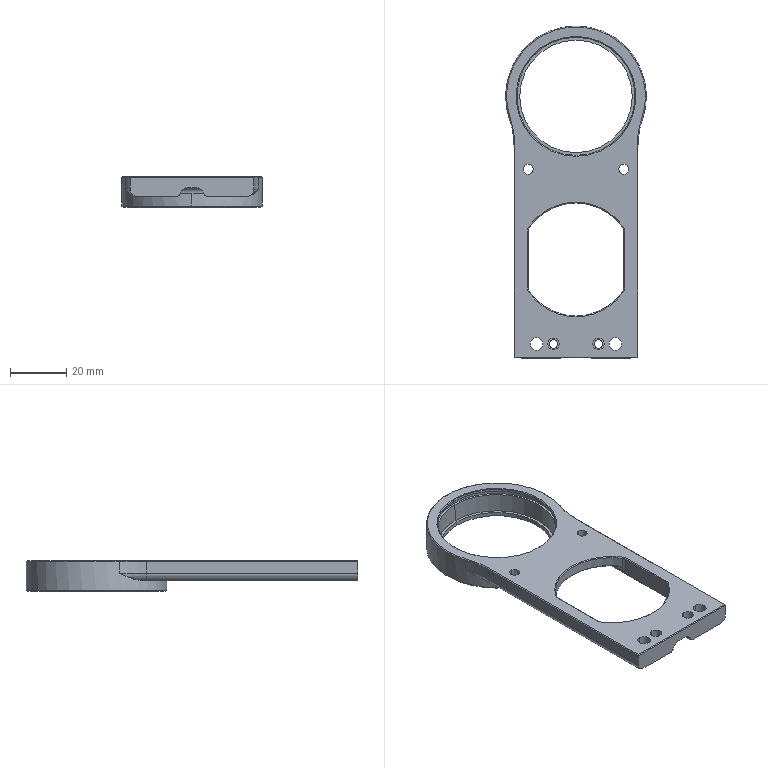NC program | NX | posted with a generic post | part box 50 x 118 x 11 mm
Lines 1 to 1102 of 9841:
N10 G17 G21 G94 G90
(FLOOR_WALL_COPY , TOOL : D80)
N12 T19 M6
N14 G54
N16 G17 G0 G90 X-45. Y0. S5000 M3
N18 G43 Z30. H19
N20 Z4.05
N22 G94 G1 Z1.05 F1200.
N24 X-40.
N26 X158.
N28 X163.
N30 Z4.05
N32 G0 Z30.
N34 X-45.
N36 Z3.1
N38 G1 Z0.1
N40 X-40.
N42 X158.
N44 X163.
N46 Z3.1
N48 G0 Z30.
(FLOOR_WALL_COPY_COPY , TOOL : D80)
N50 X-45.
N52 Z3.
N54 G1 Z0.
N56 X-40.
N58 X158.
N60 X163.
N62 Z3.
N64 G0 Z30.
N66 M5
(FLOOR_WALL_1 , TOOL : D10)
N68 T15 M6
N70 G54
N72 G17 G0 G90 X19.571 Y0. S9500 M3
N74 G43 Z30. H15
N76 Z2.5
N78 G94 G1 X19.5 Z2.496 F1000.
N80 X38.4 Z1.506
N82 X19.5 Z0.515
N84 X28.95 Z0.02
N86 X38.4 F2500.
N88 X19.5
N90 X28.95
N92 Y4.5
N94 X15.
N96 Y0.373
N98 Y-4.5
N100 X43.103
N102 G2 X43.103 Y4.5 R50.1
N104 G1 X28.95
N106 Y9.5
N108 X10.
N110 Y0.373
N112 Y-9.5
N114 X48.912
N116 G2 X48.912 Y9.5 R45.1
N118 G1 X28.95
N120 Y14.5
N122 X5.
N124 Y0.373
N126 Y-14.5
N128 X55.613
N130 G2 X55.613 Y14.5 R40.1
N132 G1 X28.95
N134 Y19.5
N136 X0.
N138 Y0.373
N140 Y-19.5
N142 X63.815
N144 G2 X63.815 Y19.5 R35.1
N146 G1 X28.95
N148 Y24.5
N150 X-5.
N152 Y-24.5
N154 X75.084
N156 G2 X75.476 Y-24.503 R27.5
N158 G1 Y-24.473
N160 G2 X75.476 Y24.473 R30.1
N162 G1 Y24.503
N164 G2 X75.084 Y24.5 R27.5
N166 G1 X28.95
N168 Z1.52
N170 G0 X19.571 Y0.
N172 G1 X19.5 Z1.516 F1000.
N174 X38.4 Z0.526
N176 X19.5 Z-0.465
N178 X28.95 Z-0.96
N180 X38.4 F2500.
N182 X19.5
N184 X28.95
N186 Y4.5
N188 X15.
N190 Y0.373
N192 Y-4.5
N194 X43.103
N196 G2 X43.103 Y4.5 R50.1
N198 G1 X28.95
N200 Y9.5
N202 X10.
N204 Y0.373
N206 Y-9.5
N208 X48.912
N210 G2 X48.912 Y9.5 R45.1
N212 G1 X28.95
N214 Y14.5
N216 X5.
N218 Y0.373
N220 Y-14.5
N222 X55.613
N224 G2 X55.613 Y14.5 R40.1
N226 G1 X28.95
N228 Y19.5
N230 X0.
N232 Y0.373
N234 Y-19.5
N236 X63.815
N238 G2 X63.815 Y19.5 R35.1
N240 G1 X28.95
N242 Y24.5
N244 X-5.
N246 Y-24.5
N248 X75.084
N250 G2 X75.476 Y-24.503 R27.5
N252 G1 Y-24.473
N254 G2 X75.476 Y24.473 R30.1
N256 G1 Y24.503
N258 G2 X75.084 Y24.5 R27.5
N260 G1 X28.95
N262 Z0.54
N264 G0 X19.571 Y0.
N266 G1 X19.5 Z0.536 F1000.
N268 X38.4 Z-0.454
N270 X19.5 Z-1.445
N272 X28.95 Z-1.94
N274 X38.4 F2500.
N276 X19.5
N278 X28.95
N280 Y4.5
N282 X15.
N284 Y0.373
N286 Y-4.5
N288 X43.103
N290 G2 X43.103 Y4.5 R50.1
N292 G1 X28.95
N294 Y9.5
N296 X10.
N298 Y0.373
N300 Y-9.5
N302 X48.912
N304 G2 X48.912 Y9.5 R45.1
N306 G1 X28.95
N308 Y14.5
N310 X5.
N312 Y0.373
N314 Y-14.5
N316 X55.613
N318 G2 X55.613 Y14.5 R40.1
N320 G1 X28.95
N322 Y19.5
N324 X0.
N326 Y0.373
N328 Y-19.5
N330 X63.815
N332 G2 X63.815 Y19.5 R35.1
N334 G1 X28.95
N336 Y24.5
N338 X-5.
N340 Y-24.5
N342 X75.084
N344 G2 X75.476 Y-24.503 R27.5
N346 G1 Y-24.473
N348 G2 X75.476 Y24.473 R30.1
N350 G1 Y24.503
N352 G2 X75.084 Y24.5 R27.5
N354 G1 X28.95
N356 Z-0.44
N358 G0 X19.571 Y0.
N360 G1 X19.5 Z-0.444 F1000.
N362 X38.4 Z-1.434
N364 X19.5 Z-2.425
N366 X28.95 Z-2.92
N368 X38.4 F2500.
N370 X19.5
N372 X28.95
N374 Y4.5
N376 X15.
N378 Y0.373
N380 Y-4.5
N382 X43.103
N384 G2 X43.103 Y4.5 R50.1
N386 G1 X28.95
N388 Y9.5
N390 X10.
N392 Y0.373
N394 Y-9.5
N396 X48.912
N398 G2 X48.912 Y9.5 R45.1
N400 G1 X28.95
N402 Y14.5
N404 X5.
N406 Y0.373
N408 Y-14.5
N410 X55.613
N412 G2 X55.613 Y14.5 R40.1
N414 G1 X28.95
N416 Y19.5
N418 X0.
N420 Y0.373
N422 Y-19.5
N424 X63.815
N426 G2 X63.815 Y19.5 R35.1
N428 G1 X28.95
N430 Y24.5
N432 X-5.
N434 Y-24.5
N436 X75.084
N438 G2 X75.476 Y-24.503 R27.5
N440 G1 Y-24.473
N442 G2 X75.476 Y24.473 R30.1
N444 G1 Y24.503
N446 G2 X75.084 Y24.5 R27.5
N448 G1 X28.95
N450 Z-1.42
N452 G0 X19.571 Y0.
N454 G1 X19.5 Z-1.424 F1000.
N456 X38.4 Z-2.414
N458 X19.5 Z-3.405
N460 X28.95 Z-3.9
N462 X38.4 F2500.
N464 X19.5
N466 X28.95
N468 Y4.5
N470 X15.
N472 Y0.373
N474 Y-4.5
N476 X43.103
N478 G2 X43.103 Y4.5 R50.1
N480 G1 X28.95
N482 Y9.5
N484 X10.
N486 Y0.373
N488 Y-9.5
N490 X48.912
N492 G2 X48.912 Y9.5 R45.1
N494 G1 X28.95
N496 Y14.5
N498 X5.
N500 Y0.373
N502 Y-14.5
N504 X55.613
N506 G2 X55.613 Y14.5 R40.1
N508 G1 X28.95
N510 Y19.5
N512 X0.
N514 Y0.373
N516 Y-19.5
N518 X63.815
N520 G2 X63.815 Y19.5 R35.1
N522 G1 X28.95
N524 Y24.5
N526 X-5.
N528 Y-24.5
N530 X75.084
N532 G2 X75.476 Y-24.503 R27.5
N534 G1 Y-24.473
N536 G2 X75.476 Y24.473 R30.1
N538 G1 Y24.503
N540 G2 X75.084 Y24.5 R27.5
N542 G1 X28.95
N544 Z-2.4
N546 G0 Z30.
(FLOOR_WALL_1_COPY , TOOL : D10)
N548 X22.071 Y8.399
N550 Z-1.8
N552 G1 X21.977 Y8.276 Z-1.808 F1000.
N554 X20.777 Y5.983 Z-1.944
N556 X19.977 Y3.522 Z-2.079
N558 X19.6 Y0.962 Z-2.215
N560 Y-0.962 Z-2.316
N562 X19.977 Y-3.522 Z-2.451
N564 X20.777 Y-5.983 Z-2.587
N566 X21.977 Y-8.276 Z-2.723
N568 X23.544 Y-10.336 Z-2.858
N570 X24.231 Y-11.009 Z-2.909
N572 X24.21 Y-11.03 Z-2.91
N574 X24.231 Y-11.009 Z-2.912
N576 X23.544 Y-10.336 Z-2.962
N578 X21.977 Y-8.276 Z-3.098
N580 X20.777 Y-5.983 Z-3.233
N582 X19.977 Y-3.522 Z-3.369
N584 X19.6 Y-0.962 Z-3.505
N586 Y0.962 Z-3.606
N588 X19.977 Y3.522 Z-3.741
N590 X20.777 Y5.983 Z-3.877
N592 X21.977 Y8.276 Z-4.012
N594 X23.544 Y10.336 Z-4.148
N596 X24.231 Y11.009 Z-4.198
N598 X24.21 Y11.03 Z-4.2
N600 X23.151 Y10.525 F2500.
N602 X17.476
N604 Y0.54
N606 X17.033 Y0.
N608 X17.475 Y-0.54
N610 X17.476 Y-10.525
N612 X23.152
N614 X24.21 Y-11.03
N616 Z-2.7
N618 G0 X22.071 Y8.399
N620 G1 X21.977 Y8.276 Z-2.708 F1000.
N622 X20.777 Y5.983 Z-2.844
N624 X19.977 Y3.522 Z-2.979
N626 X19.6 Y0.962 Z-3.115
N628 Y-0.962 Z-3.216
N630 X19.977 Y-3.522 Z-3.351
N632 X20.777 Y-5.983 Z-3.487
N634 X21.977 Y-8.276 Z-3.623
N636 X23.544 Y-10.336 Z-3.758
N638 X24.231 Y-11.009 Z-3.809
N640 X24.21 Y-11.03 Z-3.81
N642 X24.231 Y-11.009 Z-3.812
N644 X23.544 Y-10.336 Z-3.862
N646 X21.977 Y-8.276 Z-3.998
N648 X20.777 Y-5.983 Z-4.133
N650 X19.977 Y-3.522 Z-4.269
N652 X19.6 Y-0.962 Z-4.405
N654 Y0.962 Z-4.506
N656 X19.977 Y3.522 Z-4.641
N658 X20.777 Y5.983 Z-4.777
N660 X21.977 Y8.276 Z-4.912
N662 X23.544 Y10.336 Z-5.048
N664 X24.231 Y11.009 Z-5.098
N666 X24.21 Y11.03 Z-5.1
N668 X23.151 Y10.525 F2500.
N670 X17.476
N672 Y0.54
N674 X17.033 Y0.
N676 X17.475 Y-0.54
N678 X17.476 Y-10.525
N680 X23.152
N682 X24.21 Y-11.03
N684 Z-3.6
N686 G0 X22.071 Y8.399
N688 G1 X21.977 Y8.276 Z-3.608 F1000.
N690 X20.777 Y5.983 Z-3.744
N692 X19.977 Y3.522 Z-3.879
N694 X19.6 Y0.962 Z-4.015
N696 Y-0.962 Z-4.116
N698 X19.977 Y-3.522 Z-4.251
N700 X20.777 Y-5.983 Z-4.387
N702 X21.977 Y-8.276 Z-4.523
N704 X23.544 Y-10.336 Z-4.658
N706 X24.231 Y-11.009 Z-4.709
N708 X24.21 Y-11.03 Z-4.71
N710 X24.231 Y-11.009 Z-4.712
N712 X23.544 Y-10.336 Z-4.762
N714 X21.977 Y-8.276 Z-4.898
N716 X20.777 Y-5.983 Z-5.033
N718 X19.977 Y-3.522 Z-5.169
N720 X19.6 Y-0.962 Z-5.305
N722 Y0.962 Z-5.406
N724 X19.977 Y3.522 Z-5.541
N726 X20.777 Y5.983 Z-5.677
N728 X21.977 Y8.276 Z-5.812
N730 X23.544 Y10.336 Z-5.948
N732 X24.231 Y11.009 Z-5.998
N734 X24.21 Y11.03 Z-6.
N736 X23.151 Y10.525 F2500.
N738 X17.476
N740 Y0.54
N742 X17.033 Y0.
N744 X17.475 Y-0.54
N746 X17.476 Y-10.525
N748 X23.152
N750 X24.21 Y-11.03
N752 Z-4.5
N754 G0 X22.071 Y8.399
N756 G1 X21.977 Y8.276 Z-4.508 F1000.
N758 X20.777 Y5.983 Z-4.644
N760 X19.977 Y3.522 Z-4.779
N762 X19.6 Y0.962 Z-4.915
N764 Y-0.962 Z-5.016
N766 X19.977 Y-3.522 Z-5.151
N768 X20.777 Y-5.983 Z-5.287
N770 X21.977 Y-8.276 Z-5.423
N772 X23.544 Y-10.336 Z-5.558
N774 X24.231 Y-11.009 Z-5.609
N776 X24.21 Y-11.03 Z-5.61
N778 X24.231 Y-11.009 Z-5.612
N780 X23.544 Y-10.336 Z-5.662
N782 X21.977 Y-8.276 Z-5.798
N784 X20.777 Y-5.983 Z-5.933
N786 X19.977 Y-3.522 Z-6.069
N788 X19.6 Y-0.962 Z-6.205
N790 Y0.962 Z-6.306
N792 X19.977 Y3.522 Z-6.441
N794 X20.777 Y5.983 Z-6.577
N796 X21.977 Y8.276 Z-6.712
N798 X23.544 Y10.336 Z-6.848
N800 X24.231 Y11.009 Z-6.898
N802 X24.21 Y11.03 Z-6.9
N804 X23.245 Y10.569 F2500.
N806 G2 X22.705 Y9.824 R0.6
N808 G1 X21.918 Y9.769
N810 X20.677 Y9.69
N812 X19.437 Y9.685
N814 X18.332 Y9.67
N816 X18.274 Y-1.245
N818 X18.345 Y-8.645
N820 X18.337 Y-9.67
N822 X19.438 Y-9.681
N824 X20.675 Y-9.692
N826 X21.911 Y-9.752
N828 G2 X22.482 Y-10.351 R0.6
N830 G1 Y-10.525
N832 X23.152
N834 X24.21 Y-11.03
N836 Z-5.4
N838 G0 Z30.
N840 X55.564 Y-5.525
N842 Z-1.8
N844 G1 X56.332 Z-1.84 F1000.
N846 X56.597 Y-5.276 Z-1.859
N848 X56.874 Y-5.039 Z-1.878
N850 X56.67 Y-3.574 Z-1.956
N852 X56.495 Y0. Z-2.143
N854 X56.67 Y3.574 Z-2.331
N856 X56.874 Y5.039 Z-2.409
N858 X56.597 Y5.276 Z-2.428
N860 X56.332 Y5.525 Z-2.447
N862 X54.638 Z-2.535
N864 X54.937 Y4.459 Z-2.593
N866 X55.238 Y2.793 Z-2.682
N868 X55.4 Y1.107 Z-2.771
N870 Y-1.107 Z-2.887
N872 X55.238 Y-2.793 Z-2.976
N874 X54.937 Y-4.459 Z-3.064
N876 X54.638 Y-5.525 Z-3.122
N878 X56.332 Z-3.211
N880 X56.597 Y-5.276 Z-3.23
N882 X56.874 Y-5.039 Z-3.249
N884 X56.67 Y-3.574 Z-3.327
N886 X56.495 Y0. Z-3.514
N888 X56.67 Y3.574 Z-3.702
N890 X56.874 Y5.039 Z-3.78
N892 X56.597 Y5.276 Z-3.799
N894 X56.332 Y5.525 Z-3.818
N896 X54.638 Z-3.906
N898 X54.937 Y4.459 Z-3.964
N900 X55.238 Y2.793 Z-4.053
N902 X55.4 Y1.107 Z-4.142
N904 Y0. Z-4.2
N906 G2 X54.638 Y-5.525 R20.4 F2500.
N908 G1 X56.332
N910 G2 X56.874 Y-5.039 R15.725
N912 X56.874 Y5.039 R36.476
N914 X56.332 Y5.525 R15.725
N916 G1 X54.638
N918 G2 X55.4 Y0. R20.4
N920 G1 X50.4
N922 G2 X45.769 Y-11.009 R15.4
N924 G1 X45.79 Y-11.03
N926 X46.849 Y-10.525
N928 X58.533
N930 G2 X62.395 Y-7.353 R10.725
N932 X62.395 Y7.353 R31.476
N934 X58.533 Y10.525 R10.725
N936 G1 X46.848
N938 X45.79 Y11.03
N940 X45.769 Y11.009
N942 G2 X50.4 Y0. R15.4
N944 G1 Z-2.7
N946 G0 X55.564 Y-5.525
N948 G1 X56.332 Z-2.74 F1000.
N950 X56.597 Y-5.276 Z-2.759
N952 X56.874 Y-5.039 Z-2.778
N954 X56.67 Y-3.574 Z-2.856
N956 X56.495 Y0. Z-3.043
N958 X56.67 Y3.574 Z-3.231
N960 X56.874 Y5.039 Z-3.309
N962 X56.597 Y5.276 Z-3.328
N964 X56.332 Y5.525 Z-3.347
N966 X54.638 Z-3.435
N968 X54.937 Y4.459 Z-3.493
N970 X55.238 Y2.793 Z-3.582
N972 X55.4 Y1.107 Z-3.671
N974 Y-1.107 Z-3.787
N976 X55.238 Y-2.793 Z-3.876
N978 X54.937 Y-4.459 Z-3.964
N980 X54.638 Y-5.525 Z-4.022
N982 X56.332 Z-4.111
N984 X56.597 Y-5.276 Z-4.13
N986 X56.874 Y-5.039 Z-4.149
N988 X56.67 Y-3.574 Z-4.227
N990 X56.495 Y0. Z-4.414
N992 X56.67 Y3.574 Z-4.602
N994 X56.874 Y5.039 Z-4.68
N996 X56.597 Y5.276 Z-4.699
N998 X56.332 Y5.525 Z-4.718
N1000 X54.638 Z-4.806
N1002 X54.937 Y4.459 Z-4.864
N1004 X55.238 Y2.793 Z-4.953
N1006 X55.4 Y1.107 Z-5.042
N1008 Y0. Z-5.1
N1010 G2 X54.638 Y-5.525 R20.4 F2500.
N1012 G1 X56.332
N1014 G2 X56.874 Y-5.039 R15.725
N1016 X56.874 Y5.039 R36.476
N1018 X56.332 Y5.525 R15.725
N1020 G1 X54.638
N1022 G2 X55.4 Y0. R20.4
N1024 G1 X50.4
N1026 G2 X45.769 Y-11.009 R15.4
N1028 G1 X45.79 Y-11.03
N1030 X46.849 Y-10.525
N1032 X58.533
N1034 G2 X62.395 Y-7.353 R10.725
N1036 X62.395 Y7.353 R31.476
N1038 X58.533 Y10.525 R10.725
N1040 G1 X46.848
N1042 X45.79 Y11.03
N1044 X45.769 Y11.009
N1046 G2 X50.4 Y0. R15.4
N1048 G1 Z-3.6
N1050 G0 X55.564 Y-5.525
N1052 G1 X56.332 Z-3.64 F1000.
N1054 X56.597 Y-5.276 Z-3.659
N1056 X56.874 Y-5.039 Z-3.678
N1058 X56.67 Y-3.574 Z-3.756
N1060 X56.495 Y0. Z-3.943
N1062 X56.67 Y3.574 Z-4.131
N1064 X56.874 Y5.039 Z-4.209
N1066 X56.597 Y5.276 Z-4.228
N1068 X56.332 Y5.525 Z-4.247
N1070 X54.638 Z-4.335
N1072 X54.937 Y4.459 Z-4.393
N1074 X55.238 Y2.793 Z-4.482
N1076 X55.4 Y1.107 Z-4.571
N1078 Y-1.107 Z-4.687
N1080 X55.238 Y-2.793 Z-4.776
N1082 X54.937 Y-4.459 Z-4.864
N1084 X54.638 Y-5.525 Z-4.922
N1086 X56.332 Z-5.011
N1088 X56.597 Y-5.276 Z-5.03
N1090 X56.874 Y-5.039 Z-5.049
N1092 X56.67 Y-3.574 Z-5.127
N1094 X56.495 Y0. Z-5.314
N1096 X56.67 Y3.574 Z-5.502
N1098 X56.874 Y5.039 Z-5.58
N1100 X56.597 Y5.276 Z-5.599
N1102 X56.332 Y5.525 Z-5.618
N1104 X54.638 Z-5.706
N1106 X54.937 Y4.459 Z-5.764
N1108 X55.238 Y2.793 Z-5.853
N1110 X55.4 Y1.107 Z-5.942
N1112 Y0. Z-6.
N1114 G2 X54.638 Y-5.525 R20.4 F2500.
N1116 G1 X56.332
N1118 G2 X56.874 Y-5.039 R15.725
N1120 X56.874 Y5.039 R36.476
N1122 X56.332 Y5.525 R15.725
N1124 G1 X54.638
N1126 G2 X55.4 Y0. R20.4
N1128 G1 X50.4
N1130 G2 X45.769 Y-11.009 R15.4
N1132 G1 X45.79 Y-11.03
N1134 X46.849 Y-10.525
N1136 X58.533
N1138 G2 X62.395 Y-7.353 R10.725
N1140 X62.395 Y7.353 R31.476
N1142 X58.533 Y10.525 R10.725
N1144 G1 X46.848
N1146 X45.79 Y11.03
N1148 X45.769 Y11.009
N1150 G2 X50.4 Y0. R15.4
N1152 G1 Z-4.5
N1154 G0 X55.153 Y3.218
N1156 G1 X55.4 Y1.111 Z-4.611 F1000.
N1158 Y-1.102 Z-4.727
N1160 X55.107 Y-3.617 Z-4.86
N1162 X54.853 Y-4.694 Z-4.918
N1164 X55.316 Y-4.692 Z-4.942
N1166 X56.034 Y-4.691 Z-4.98
N1168 X56.221 Y-4.509 Z-4.993
N1170 X56.189 Y-4.075 Z-5.016
N1172 X56.013 Y-1.428 Z-5.155
N1174 X56.047 Y4.631 Z-5.473
N1176 X55.798 Y4.696 Z-5.486
N1178 X55.293 Y4.699 Z-5.513
N1180 X54.851 Y4.702 Z-5.536
N1182 X55.106 Y3.625 Z-5.594
N1184 X55.4 Y1.111 Z-5.727
N1186 Y-1.102 Z-5.843
N1188 X55.107 Y-3.617 Z-5.975
N1190 X54.853 Y-4.694 Z-6.033
N1192 X55.316 Y-4.692 Z-6.058
N1194 X56.034 Y-4.691 Z-6.095
N1196 X56.221 Y-4.509 Z-6.109
N1198 X56.189 Y-4.075 Z-6.132
N1200 X56.013 Y-1.428 Z-6.271
N1202 X56.047 Y4.631 Z-6.588
N1204 X55.798 Y4.696 Z-6.602
N1206 X55.293 Y4.699 Z-6.628
N1208 X54.851 Y4.702 Z-6.651
N1210 X55.106 Y3.625 Z-6.709
N1212 X55.4 Y1.111 Z-6.842
N1214 Y0.004 Z-6.9
N1216 G2 X54.853 Y-4.694 R20.4 F2500.
N1218 G1 X55.316 Y-4.692
N1220 X56.034 Y-4.691
N1222 X56.221 Y-4.509
N1224 X56.189 Y-4.075
N1226 X56.013 Y-1.428
N1228 X56.047 Y4.631
N1230 X55.798 Y4.696
N1232 X55.293 Y4.699
N1234 X54.851 Y4.702
N1236 G2 X55.4 Y0.004 R20.4
N1238 G1 X50.4 Y0.003
N1240 G2 X45.769 Y-11.009 R15.4
N1242 G1 X45.79 Y-11.03
N1244 X46.849 Y-10.525
N1246 X47.494
N1248 Y-10.322
N1250 G2 X48.09 Y-9.722 R0.6
N1252 G1 X56.508 Y-9.69
N1254 X57.672 Y-9.572
N1256 X58.304 Y-9.508
N1258 X61.375 Y-6.445
N1260 X61.013 Y-1.259
N1262 X61.054 Y4.978
N1264 X61.305 Y6.253
N1266 X61.426 Y6.866
N1268 X59.822 Y8.056
N1270 X59.661 Y8.187
N1272 X58.687 Y9.056
N1274 X57.499 Y9.419
N1276 X56.459 Y9.691
N1278 X48.09 Y9.744
N1280 G2 X47.494 Y10.344 R0.6
N1282 G1 Y10.525
N1284 X46.848
N1286 X45.79 Y11.03
N1288 X45.769 Y11.009
N1290 G2 X50.4 Y0.003 R15.4
N1292 G1 Z-5.4
N1294 G0 Z30.
N1296 M5
(FLOOR_WALL_1_COPY_1_COPY_COPY , TOOL : D10JING)
N1298 T14 M6
N1300 G54
N1302 G17 G0 G90 X-8. Y-0.373 S9500 M3
N1304 G43 Z30. H14
N1306 Z-3.
N1308 G94 G1 Z-4. F1000.
N1310 X-5.
N1312 X15.7 F1200.
N1314 Y-4.155
N1316 X-5.
N1318 Y-7.936
N1320 X15.7
N1322 Y-12.
N1324 G3 X16. Y-12.3 R0.3
N1326 G1 X59.467
N1328 G2 X63.764 Y-8.688 R8.95
N1330 G3 X64.841 Y-11.718 R30.5
N1332 G1 X-5.
N1334 Y-15.5
N1336 X66.732
N1338 G3 X69.368 Y-19.282 R30.5
N1340 G1 X-5.
N1342 Y-23.063
N1344 X73.042
N1346 Z-3.
N1348 G0 X77.927 Y-26.515
N1350 G1 Z-4. F1000.
N1352 X78.1 Y-26.211
N1354 X75.653 Y-24.476
N1356 G2 X64.234 Y-8.516 R30. F1200.
N1358 G1 X63.382 Y-5.639
N1360 X63.038 Y-5.705
N1362 Z-3.
N1364 G0 Z30.
N1366 X23.193 Y9.089
N1368 Z-6.
N1370 G1 Z-7. F1000.
N1372 X22.66 Y9.5
N1374 Y-9.5 F1200.
N1376 X18.5
N1378 Y9.5
N1380 Z-6.
N1382 G0 Z30.
N1384 X24.592 Y10.671
N1386 Z-6.
N1388 G1 Z-7. F1000.
N1390 X24.167 Y10.988
N1392 X22.703 Y10. F1200.
N1394 X18.
N1396 Y-10.
N1398 X22.663
N1400 X24.153 Y-10.974
N1402 X24.572 Y-10.651
N1404 Z-6.
N1406 G0 Z30.
N1408 X-8. Y24.5
N1410 Z-3.
N1412 G1 Z-4. F1000.
N1414 X-5.
N1416 X74.834 F1200.
N1418 G3 X70.617 Y20.718 R30.5
N1420 G1 X-5.
N1422 Y16.936
N1424 X67.635
N1426 G3 X65.483 Y13.155 R30.5
N1428 G1 X-5.
N1430 Y9.373
N1432 X15.7
N1434 X18.7
N1436 Z-3.
N1438 G0 X63.038 Y5.705
N1440 G1 Z-4. F1000.
N1442 X63.382 Y5.639
N1444 X64.234 Y8.516
N1446 G2 X75.653 Y24.476 R30. F1200.
N1448 G1 X78.1 Y26.211
N1450 X77.927 Y26.515
N1452 Z-3.
N1454 G0 Z30.
N1456 X44.123 Y9.497
N1458 Z-6.
N1460 G1 Z-7. F1000.
N1462 X47.123
N1464 X58.041 F1200.
N1466 G3 X61.223 Y6.816 R11.75
N1468 X60.849 Y4.748 R32.5
N1470 G1 X49.65
N1472 X50.4 Y-0.001
N1474 X60.5
N1476 G3 X60.849 Y-4.751 R32.5
N1478 G1 X49.649
N1480 X47.121 Y-9.5
N1482 X58.039
N1484 Z-6.
N1486 G0 Z30.
N1488 X45.409 Y-10.671
N1490 Z-6.
N1492 G1 Z-7. F1000.
N1494 X45.833 Y-10.988
N1496 X47.298 Y-10. F1200.
N1498 X58.277
N1500 G2 X61.791 Y-7.072 R11.25
N1502 X61.791 Y7.072 R32.
N1504 X58.277 Y10. R11.25
N1506 G1 X47.338
N1508 X45.848 Y10.973
N1510 X45.428 Y10.65
N1512 Z-6.
N1514 G0 Z30.
N1516 M5
(HOLE_MILLING_2 , TOOL : D4)
N1518 T11 M6
N1520 G54
N1522 G17 G0 G90 X5. Y14. S9500 M3
N1524 G43 Z30. H11
N1526 Z-3.5
N1528 G94 G3 X5.75 Y14.75 R0.75 F1250.
N1530 X5. Y15.5 R0.75
N1532 X5. Y15.5 Z-3.9 I0. J-1.5
N1534 X5. Y15.5 Z-4.3 I0. J-1.5
N1536 X5. Y15.5 Z-4.7 I0. J-1.5
N1538 X5. Y15.5 Z-5.1 I0. J-1.5
N1540 X5. Y15.5 Z-5.5 I0. J-1.5
N1542 X5. Y15.5 Z-5.9 I0. J-1.5
N1544 X5. Y15.5 Z-6.3 I0. J-1.5
N1546 X5. Y15.5 Z-6.7 I0. J-1.5
N1548 X5. Y15.5 Z-7.1 I0. J-1.5
N1550 X6.5 Y14. Z-7.4 R-1.5
N1552 X5. Y15.5 R1.5
N1554 X6.5 Y14. R-1.5
N1556 X5.75 Y14.75 R0.75
N1558 X5. Y14. R0.75
N1560 G0 Z30.
N1562 Y-14.
N1564 Z-3.5
N1566 G3 X5.75 Y-13.25 R0.75
N1568 X5. Y-12.5 R0.75
N1570 X5. Y-12.5 Z-3.9 I0. J-1.5
N1572 X5. Y-12.5 Z-4.3 I0. J-1.5
N1574 X5. Y-12.5 Z-4.7 I0. J-1.5
N1576 X5. Y-12.5 Z-5.1 I0. J-1.5
N1578 X5. Y-12.5 Z-5.5 I0. J-1.5
N1580 X5. Y-12.5 Z-5.9 I0. J-1.5
N1582 X5. Y-12.5 Z-6.3 I0. J-1.5
N1584 X5. Y-12.5 Z-6.7 I0. J-1.5
N1586 X5. Y-12.5 Z-7.1 I0. J-1.5
N1588 X6.5 Y-14. Z-7.4 R-1.5
N1590 X5. Y-12.5 R1.5
N1592 X6.5 Y-14. R-1.5
N1594 X5.75 Y-13.25 R0.75
N1596 X5. Y-14. R0.75
N1598 G0 Z30.
(FLOOR_WALL_1_COPY_1 , TOOL : D4)
N1600 X17.284 Y-5.035
N1602 Z-1.8
N1604 G1 X17.209 Y-4.81 Z-1.812 F1000.
N1606 X16.807 Y-2.946 Z-1.912
N1608 X16.6 Y-1.051 Z-2.012
N1610 Y1.051 Z-2.122
N1612 X16.825 Y3.054 Z-2.228
N1614 X17.267 Y5.021 Z-2.334
N1616 X17.611 Y6.014 Z-2.389
N1618 X14.476 Y6.166 Z-2.553
N1620 Y1.613 Z-2.792
N1622 X13.956 Y0.979 Z-2.835
N1624 X13.291 Y0.168 Z-2.89
N1626 X-2. Z-3.691
N1628 Y0. Z-3.7
N1630 Y-0.168 F2000.
N1632 X13.291
N1634 X13.965 Y-0.99
N1636 X14.475 Y-1.613
N1638 X14.476 Y-5.952
N1640 X17.54 Y-5.807
N1642 G2 X17.611 Y6.014 R18.4
N1644 G1 X14.476 Y6.166
N1646 Y1.613
N1648 X13.956 Y0.979
N1650 X13.291 Y0.168
N1652 X-2.
N1654 Y0.
N1656 Z-2.2
N1658 G0 Z30.
N1660 X17.284 Y-5.035
N1662 Z-2.2
N1664 G1 X17.209 Y-4.81 Z-2.212 F1000.
N1666 X16.807 Y-2.946 Z-2.312
N1668 X16.6 Y-1.051 Z-2.412
N1670 Y1.051 Z-2.522
N1672 X16.825 Y3.054 Z-2.628
N1674 X17.267 Y5.021 Z-2.734
N1676 X17.611 Y6.014 Z-2.789
N1678 X14.476 Y6.166 Z-2.953
N1680 Y1.613 Z-3.192
N1682 X13.956 Y0.979 Z-3.235
N1684 X13.291 Y0.168 Z-3.29
N1686 X-2. Z-4.091
N1688 Y0. Z-4.1
N1690 Y-0.168 F2000.
N1692 X13.291
N1694 X13.965 Y-0.99
N1696 X14.475 Y-1.613
N1698 X14.476 Y-5.952
N1700 X17.54 Y-5.807
N1702 G2 X17.611 Y6.014 R18.4
N1704 G1 X14.476 Y6.166
N1706 Y1.613
N1708 X13.956 Y0.979
N1710 X13.291 Y0.168
N1712 X-2.
N1714 Y0.
N1716 Z-2.6
N1718 G0 Z30.
N1720 X17.284 Y-5.035
N1722 Z-2.6
N1724 G1 X17.209 Y-4.81 Z-2.612 F1000.
N1726 X16.807 Y-2.946 Z-2.712
N1728 X16.6 Y-1.051 Z-2.812
N1730 Y1.051 Z-2.922
N1732 X16.825 Y3.054 Z-3.028
N1734 X17.267 Y5.021 Z-3.134
N1736 X17.611 Y6.014 Z-3.189
N1738 X14.476 Y6.166 Z-3.353
N1740 Y1.613 Z-3.592
N1742 X13.956 Y0.979 Z-3.635
N1744 X13.291 Y0.168 Z-3.69
N1746 X-2. Z-4.491
N1748 Y0. Z-4.5
N1750 Y-0.168 F2000.
N1752 X13.291
N1754 X13.965 Y-0.99
N1756 X14.475 Y-1.613
N1758 X14.476 Y-5.952
N1760 X17.54 Y-5.807
N1762 G2 X17.611 Y6.014 R18.4
N1764 G1 X14.476 Y6.166
N1766 Y1.613
N1768 X13.956 Y0.979
N1770 X13.291 Y0.168
N1772 X-2.
N1774 Y0.
N1776 Z-3.
N1778 G0 Z30.
N1780 X17.284 Y-5.035
N1782 Z-3.
N1784 G1 X17.209 Y-4.81 Z-3.012 F1000.
N1786 X16.807 Y-2.946 Z-3.112
N1788 X16.6 Y-1.051 Z-3.212
N1790 Y1.051 Z-3.322
N1792 X16.825 Y3.054 Z-3.428
N1794 X17.267 Y5.021 Z-3.534
N1796 X17.611 Y6.014 Z-3.589
N1798 X14.476 Y6.166 Z-3.753
N1800 Y1.613 Z-3.992
N1802 X13.956 Y0.979 Z-4.035
N1804 X13.291 Y0.168 Z-4.09
N1806 X-2. Z-4.891
N1808 Y0. Z-4.9
N1810 Y-0.168 F2000.
N1812 X13.291
N1814 X13.965 Y-0.99
N1816 X14.475 Y-1.613
N1818 X14.476 Y-5.952
N1820 X17.54 Y-5.807
N1822 G2 X17.611 Y6.014 R18.4
N1824 G1 X14.476 Y6.166
N1826 Y1.613
N1828 X13.956 Y0.979
N1830 X13.291 Y0.168
N1832 X-2.
N1834 Y0.
N1836 Z-3.4
N1838 G0 Z30.
N1840 X17.284 Y-5.035
N1842 Z-3.4
N1844 G1 X17.209 Y-4.81 Z-3.412 F1000.
N1846 X16.807 Y-2.946 Z-3.512
N1848 X16.6 Y-1.051 Z-3.612
N1850 Y1.051 Z-3.722
N1852 X16.825 Y3.054 Z-3.828
N1854 X17.267 Y5.021 Z-3.934
N1856 X17.611 Y6.014 Z-3.989
N1858 X14.476 Y6.166 Z-4.153
N1860 Y1.613 Z-4.392
N1862 X13.956 Y0.979 Z-4.435
N1864 X13.291 Y0.168 Z-4.49
N1866 X-2. Z-5.291
N1868 Y0. Z-5.3
N1870 Y-0.168 F2000.
N1872 X13.291
N1874 X13.965 Y-0.99
N1876 X14.475 Y-1.613
N1878 X14.476 Y-5.952
N1880 X17.54 Y-5.807
N1882 G2 X17.611 Y6.014 R18.4
N1884 G1 X14.476 Y6.166
N1886 Y1.613
N1888 X13.956 Y0.979
N1890 X13.291 Y0.168
N1892 X-2.
N1894 Y0.
N1896 Z-3.8
N1898 G0 Z30.
N1900 X17.284 Y-5.035
N1902 Z-3.8
N1904 G1 X17.209 Y-4.81 Z-3.812 F1000.
N1906 X16.807 Y-2.946 Z-3.912
N1908 X16.6 Y-1.051 Z-4.012
N1910 Y1.051 Z-4.122
N1912 X16.825 Y3.054 Z-4.228
N1914 X17.267 Y5.021 Z-4.334
N1916 X17.611 Y6.014 Z-4.389
N1918 X14.476 Y6.166 Z-4.553
N1920 Y1.613 Z-4.792
N1922 X13.956 Y0.979 Z-4.835
N1924 X13.291 Y0.168 Z-4.89
N1926 X-2. Z-5.691
N1928 Y0. Z-5.7
N1930 Y-0.168 F2000.
N1932 X13.291
N1934 X13.965 Y-0.99
N1936 X14.475 Y-1.613
N1938 X14.476 Y-5.952
N1940 X17.54 Y-5.807
N1942 G2 X17.611 Y6.014 R18.4
N1944 G1 X14.476 Y6.166
N1946 Y1.613
N1948 X13.956 Y0.979
N1950 X13.291 Y0.168
N1952 X-2.
N1954 Y0.
N1956 Z-4.2
N1958 G0 Z30.
N1960 X17.284 Y-5.035
N1962 Z-4.2
N1964 G1 X17.209 Y-4.81 Z-4.212 F1000.
N1966 X16.807 Y-2.946 Z-4.312
N1968 X16.6 Y-1.051 Z-4.412
N1970 Y1.051 Z-4.522
N1972 X16.825 Y3.054 Z-4.628
N1974 X17.267 Y5.021 Z-4.734
N1976 X17.611 Y6.014 Z-4.789
N1978 X14.476 Y6.166 Z-4.953
N1980 Y1.613 Z-5.192
N1982 X13.956 Y0.979 Z-5.235
N1984 X13.291 Y0.168 Z-5.29
N1986 X-2. Z-6.091
N1988 Y0. Z-6.1
N1990 Y-0.168 F2000.
N1992 X13.291
N1994 X13.965 Y-0.99
N1996 X14.475 Y-1.613
N1998 X14.476 Y-5.952
N2000 X17.54 Y-5.807
N2002 G2 X17.611 Y6.014 R18.4
N2004 G1 X14.476 Y6.166
N2006 Y1.613
N2008 X13.956 Y0.979
N2010 X13.291 Y0.168
N2012 X-2.
N2014 Y0.
N2016 Z-4.6
N2018 G0 Z30.
N2020 X17.284 Y-5.035
N2022 Z-4.6
N2024 G1 X17.209 Y-4.81 Z-4.612 F1000.
N2026 X16.807 Y-2.946 Z-4.712
N2028 X16.6 Y-1.051 Z-4.812
N2030 Y1.051 Z-4.922
N2032 X16.825 Y3.054 Z-5.028
N2034 X17.267 Y5.021 Z-5.134
N2036 X17.611 Y6.014 Z-5.189
N2038 X14.476 Y6.166 Z-5.353
N2040 Y1.613 Z-5.592
N2042 X13.956 Y0.979 Z-5.635
N2044 X13.291 Y0.168 Z-5.69
N2046 X-2. Z-6.491
N2048 Y0. Z-6.5
N2050 Y-0.168 F2000.
N2052 X13.291
N2054 X13.965 Y-0.99
N2056 X14.475 Y-1.613
N2058 X14.476 Y-5.952
N2060 X17.54 Y-5.807
N2062 G2 X17.611 Y6.014 R18.4
N2064 G1 X14.476 Y6.166
N2066 Y1.613
N2068 X13.956 Y0.979
N2070 X13.291 Y0.168
N2072 X-2.
N2074 Y0.
N2076 Z-5.
N2078 G0 Z30.
N2080 X16.802 Y2.847
N2082 Z-5.
N2084 G1 X16.825 Y3.054 Z-5.011 F1000.
N2086 X17.267 Y5.021 Z-5.117
N2088 X17.611 Y6.014 Z-5.172
N2090 X14.476 Y6.166 Z-5.336
N2092 Y5.776 Z-5.357
N2094 X14.842 Z-5.376
N2096 X15.172 Y5.433 Z-5.401
N2098 X15.1 Y3.538 Z-5.5
N2100 X14.888 Y1.334 Z-5.616
N2102 X14.626 Y-0.366 Z-5.706
N2104 X14.834 Y-1.306 Z-5.757
N2106 X15.089 Y-4.145 Z-5.906
N2108 X15.145 Y-5.268 Z-5.965
N2110 X14.812 Y-5.617 Z-5.99
N2112 X14.476 Z-6.008
N2114 Y-5.952 Z-6.026
N2116 X17.54 Y-5.807 Z-6.186
N2118 X17.209 Y-4.81 Z-6.241
N2120 X16.807 Y-2.946 Z-6.341
N2122 X16.6 Y-1.051 Z-6.441
N2124 Y1.051 Z-6.551
N2126 X16.825 Y3.054 Z-6.657
N2128 X17.267 Y5.021 Z-6.763
N2130 X17.611 Y6.014 Z-6.818
N2132 X16.043 Y6.09 Z-6.9
N2134 X14.476 Y6.166 F2000.
N2136 Y5.776
N2138 X14.666
N2140 G2 X15.166 Y5.257 R0.5
N2142 X14.626 Y-0.366 R49.275
N2144 G1 X14.834 Y-1.306
N2146 X15.089 Y-4.145
N2148 X15.136 Y-5.093
N2150 G2 X14.637 Y-5.617 R0.5
N2152 G1 X14.476
N2154 Y-5.952
N2156 X17.54 Y-5.807
N2158 G2 X17.611 Y6.014 R18.4
N2160 G1 X16.043 Y6.09
N2162 Z-5.4
N2164 G0 Z30.
N2166 M5